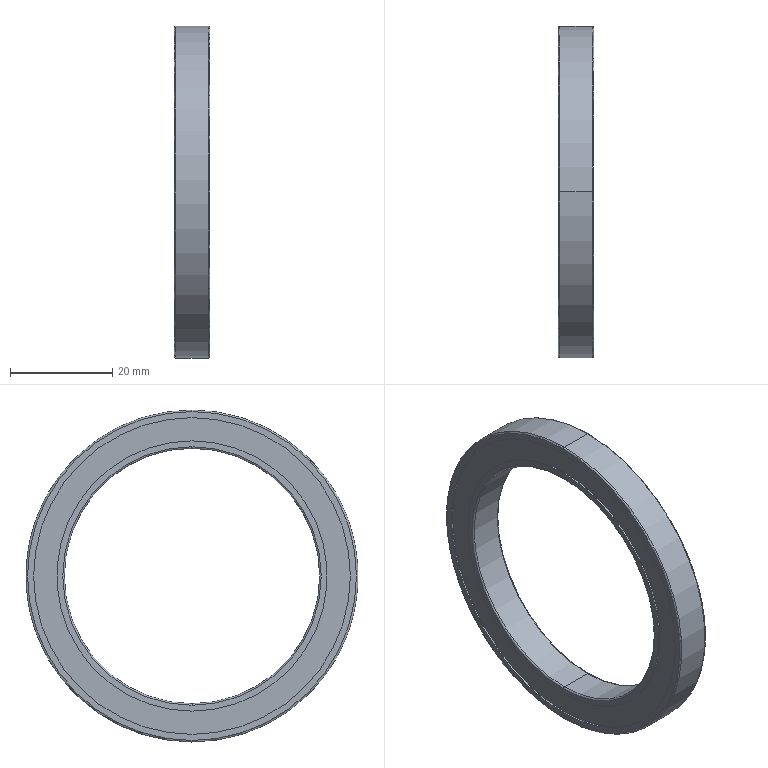Part | SolidWorks | features Fillet 2, Revolution 1 | 1 solid | 26 faces | box 7 x 65 x 65 mm | volume 8944 mm3 | cylinder 12 | torus 8 | plane 6 | commonest cylinder face diameters 52.9 x4 62 x4 50 x2 65 x2
STEP:
#1=CARTESIAN_POINT('',(0.3,0.,25.));
#2=VERTEX_POINT('',#1);
#3=CARTESIAN_POINT('',(0.3,0.,-25.));
#4=VERTEX_POINT('',#3);
#5=CARTESIAN_POINT('',(0.3,0.,0.));
#6=DIRECTION('',(-1.,0.,0.));
#7=DIRECTION('',(0.,0.,-1.));
#8=AXIS2_PLACEMENT_3D('',#5,#6,#7);
#9=CIRCLE('',#8,25.);
#10=EDGE_CURVE('',#2,#4,#9,.T.);
#11=ORIENTED_EDGE('',*,*,#10,.F.);
#12=CARTESIAN_POINT('',(0.,0.,25.3));
#13=VERTEX_POINT('',#12);
#14=CARTESIAN_POINT('',(0.3,0.,25.3));
#15=DIRECTION('',(0.,1.,0.));
#16=DIRECTION('',(0.,0.,1.));
#17=AXIS2_PLACEMENT_3D('',#14,#15,#16);
#18=CIRCLE('',#17,0.3);
#19=EDGE_CURVE('',#2,#13,#18,.T.);
#20=ORIENTED_EDGE('',*,*,#19,.T.);
#21=CARTESIAN_POINT('',(0.,0.,-25.3));
#22=VERTEX_POINT('',#21);
#23=CARTESIAN_POINT('',(0.,0.,0.));
#24=DIRECTION('',(1.,0.,0.));
#25=DIRECTION('',(0.,0.,-1.));
#26=AXIS2_PLACEMENT_3D('',#23,#24,#25);
#27=CIRCLE('',#26,25.3);
#28=EDGE_CURVE('',#22,#13,#27,.T.);
#29=ORIENTED_EDGE('',*,*,#28,.F.);
#30=CARTESIAN_POINT('',(0.3,0.,-25.3));
#31=DIRECTION('',(0.,-1.,0.));
#32=DIRECTION('',(0.,0.,-1.));
#33=AXIS2_PLACEMENT_3D('',#30,#31,#32);
#34=CIRCLE('',#33,0.3);
#35=EDGE_CURVE('',#4,#22,#34,.T.);
#36=ORIENTED_EDGE('',*,*,#35,.F.);
#37=EDGE_LOOP('',(#11,#20,#29,#36));
#38=FACE_OUTER_BOUND('',#37,.T.);
#39=CARTESIAN_POINT('',(0.3,0.,0.));
#40=DIRECTION('',(1.,0.,0.));
#41=DIRECTION('',(0.,0.,-1.));
#42=AXIS2_PLACEMENT_3D('',#39,#40,#41);
#43=TOROIDAL_SURFACE('',#42,25.3,0.3);
#44=ADVANCED_FACE('',(#38),#43,.T.);
#45=CARTESIAN_POINT('',(6.7,0.,-25.));
#46=VERTEX_POINT('',#45);
#47=CARTESIAN_POINT('',(6.7,0.,25.));
#48=VERTEX_POINT('',#47);
#49=CARTESIAN_POINT('',(6.7,0.,0.));
#50=DIRECTION('',(1.,0.,0.));
#51=DIRECTION('',(0.,0.,1.));
#52=AXIS2_PLACEMENT_3D('',#49,#50,#51);
#53=CIRCLE('',#52,25.);
#54=EDGE_CURVE('',#46,#48,#53,.T.);
#55=ORIENTED_EDGE('',*,*,#54,.F.);
#56=CARTESIAN_POINT('',(7.,0.,-25.3));
#57=VERTEX_POINT('',#56);
#58=CARTESIAN_POINT('',(6.7,0.,-25.3));
#59=DIRECTION('',(0.,1.,0.));
#60=DIRECTION('',(0.,0.,1.));
#61=AXIS2_PLACEMENT_3D('',#58,#59,#60);
#62=CIRCLE('',#61,0.3);
#63=EDGE_CURVE('',#46,#57,#62,.T.);
#64=ORIENTED_EDGE('',*,*,#63,.T.);
#65=CARTESIAN_POINT('',(7.,0.,25.3));
#66=VERTEX_POINT('',#65);
#67=CARTESIAN_POINT('',(7.,0.,0.));
#68=DIRECTION('',(-1.,0.,0.));
#69=DIRECTION('',(0.,0.,1.));
#70=AXIS2_PLACEMENT_3D('',#67,#68,#69);
#71=CIRCLE('',#70,25.3);
#72=EDGE_CURVE('',#66,#57,#71,.T.);
#73=ORIENTED_EDGE('',*,*,#72,.F.);
#74=CARTESIAN_POINT('',(6.7,0.,25.3));
#75=DIRECTION('',(0.,-1.,0.));
#76=DIRECTION('',(0.,0.,-1.));
#77=AXIS2_PLACEMENT_3D('',#74,#75,#76);
#78=CIRCLE('',#77,0.3);
#79=EDGE_CURVE('',#48,#66,#78,.T.);
#80=ORIENTED_EDGE('',*,*,#79,.F.);
#81=EDGE_LOOP('',(#55,#64,#73,#80));
#82=FACE_OUTER_BOUND('',#81,.T.);
#83=CARTESIAN_POINT('',(6.7,0.,0.));
#84=DIRECTION('',(-1.,0.,0.));
#85=DIRECTION('',(0.,0.,1.));
#86=AXIS2_PLACEMENT_3D('',#83,#84,#85);
#87=TOROIDAL_SURFACE('',#86,25.3,0.3);
#88=ADVANCED_FACE('',(#82),#87,.T.);
#89=CARTESIAN_POINT('',(0.,0.,32.2));
#90=VERTEX_POINT('',#89);
#91=CARTESIAN_POINT('',(0.,0.,-32.2));
#92=VERTEX_POINT('',#91);
#93=CARTESIAN_POINT('',(0.,0.,0.));
#94=DIRECTION('',(-1.,0.,0.));
#95=DIRECTION('',(0.,0.,-1.));
#96=AXIS2_PLACEMENT_3D('',#93,#94,#95);
#97=CIRCLE('',#96,32.2);
#98=EDGE_CURVE('',#90,#92,#97,.T.);
#99=ORIENTED_EDGE('',*,*,#98,.F.);
#100=CARTESIAN_POINT('',(0.3,0.,32.5));
#101=VERTEX_POINT('',#100);
#102=CARTESIAN_POINT('',(0.3,0.,32.2));
#103=DIRECTION('',(0.,1.,0.));
#104=DIRECTION('',(0.,0.,1.));
#105=AXIS2_PLACEMENT_3D('',#102,#103,#104);
#106=CIRCLE('',#105,0.3);
#107=EDGE_CURVE('',#90,#101,#106,.T.);
#108=ORIENTED_EDGE('',*,*,#107,.T.);
#109=CARTESIAN_POINT('',(0.3,0.,-32.5));
#110=VERTEX_POINT('',#109);
#111=CARTESIAN_POINT('',(0.3,0.,0.));
#112=DIRECTION('',(1.,0.,0.));
#113=DIRECTION('',(0.,0.,-1.));
#114=AXIS2_PLACEMENT_3D('',#111,#112,#113);
#115=CIRCLE('',#114,32.5);
#116=EDGE_CURVE('',#110,#101,#115,.T.);
#117=ORIENTED_EDGE('',*,*,#116,.F.);
#118=CARTESIAN_POINT('',(0.3,0.,-32.2));
#119=DIRECTION('',(0.,-1.,0.));
#120=DIRECTION('',(0.,0.,-1.));
#121=AXIS2_PLACEMENT_3D('',#118,#119,#120);
#122=CIRCLE('',#121,0.3);
#123=EDGE_CURVE('',#92,#110,#122,.T.);
#124=ORIENTED_EDGE('',*,*,#123,.F.);
#125=EDGE_LOOP('',(#99,#108,#117,#124));
#126=FACE_OUTER_BOUND('',#125,.T.);
#127=CARTESIAN_POINT('',(0.3,0.,0.));
#128=DIRECTION('',(1.,0.,0.));
#129=DIRECTION('',(0.,0.,-1.));
#130=AXIS2_PLACEMENT_3D('',#127,#128,#129);
#131=TOROIDAL_SURFACE('',#130,32.2,0.3);
#132=ADVANCED_FACE('',(#126),#131,.T.);
#133=CARTESIAN_POINT('',(7.,0.,-32.2));
#134=VERTEX_POINT('',#133);
#135=CARTESIAN_POINT('',(7.,0.,32.2));
#136=VERTEX_POINT('',#135);
#137=CARTESIAN_POINT('',(7.,0.,0.));
#138=DIRECTION('',(1.,0.,0.));
#139=DIRECTION('',(0.,0.,1.));
#140=AXIS2_PLACEMENT_3D('',#137,#138,#139);
#141=CIRCLE('',#140,32.2);
#142=EDGE_CURVE('',#134,#136,#141,.T.);
#143=ORIENTED_EDGE('',*,*,#142,.F.);
#144=CARTESIAN_POINT('',(6.7,0.,-32.5));
#145=VERTEX_POINT('',#144);
#146=CARTESIAN_POINT('',(6.7,0.,-32.2));
#147=DIRECTION('',(0.,1.,0.));
#148=DIRECTION('',(0.,0.,1.));
#149=AXIS2_PLACEMENT_3D('',#146,#147,#148);
#150=CIRCLE('',#149,0.3);
#151=EDGE_CURVE('',#134,#145,#150,.T.);
#152=ORIENTED_EDGE('',*,*,#151,.T.);
#153=CARTESIAN_POINT('',(6.7,0.,32.5));
#154=VERTEX_POINT('',#153);
#155=CARTESIAN_POINT('',(6.7,0.,0.));
#156=DIRECTION('',(-1.,0.,0.));
#157=DIRECTION('',(0.,0.,1.));
#158=AXIS2_PLACEMENT_3D('',#155,#156,#157);
#159=CIRCLE('',#158,32.5);
#160=EDGE_CURVE('',#154,#145,#159,.T.);
#161=ORIENTED_EDGE('',*,*,#160,.F.);
#162=CARTESIAN_POINT('',(6.7,0.,32.2));
#163=DIRECTION('',(0.,-1.,0.));
#164=DIRECTION('',(0.,0.,-1.));
#165=AXIS2_PLACEMENT_3D('',#162,#163,#164);
#166=CIRCLE('',#165,0.3);
#167=EDGE_CURVE('',#136,#154,#166,.T.);
#168=ORIENTED_EDGE('',*,*,#167,.F.);
#169=EDGE_LOOP('',(#143,#152,#161,#168));
#170=FACE_OUTER_BOUND('',#169,.T.);
#171=CARTESIAN_POINT('',(6.7,0.,0.));
#172=DIRECTION('',(-1.,0.,0.));
#173=DIRECTION('',(0.,0.,1.));
#174=AXIS2_PLACEMENT_3D('',#171,#172,#173);
#175=TOROIDAL_SURFACE('',#174,32.2,0.3);
#176=ADVANCED_FACE('',(#170),#175,.T.);
#177=ORIENTED_EDGE('',*,*,#160,.T.);
#178=CARTESIAN_POINT('',(0.,0.,-32.5));
#179=DIRECTION('',(-1.,0.,0.));
#180=VECTOR('',#179,1000.);
#181=LINE('',#178,#180);
#182=EDGE_CURVE('',#145,#110,#181,.T.);
#183=ORIENTED_EDGE('',*,*,#182,.T.);
#184=ORIENTED_EDGE('',*,*,#116,.T.);
#185=CARTESIAN_POINT('',(0.,0.,32.5));
#186=DIRECTION('',(-1.,0.,0.));
#187=VECTOR('',#186,1000.);
#188=LINE('',#185,#187);
#189=EDGE_CURVE('',#154,#101,#188,.T.);
#190=ORIENTED_EDGE('',*,*,#189,.F.);
#191=EDGE_LOOP('',(#177,#183,#184,#190));
#192=FACE_OUTER_BOUND('',#191,.T.);
#193=CARTESIAN_POINT('',(0.,0.,0.));
#194=DIRECTION('',(-1.,0.,0.));
#195=DIRECTION('',(0.,0.,1.));
#196=AXIS2_PLACEMENT_3D('',#193,#194,#195);
#197=CYLINDRICAL_SURFACE('',#196,32.5);
#198=ADVANCED_FACE('',(#192),#197,.T.);
#199=CARTESIAN_POINT('',(7.,0.,-31.));
#200=VERTEX_POINT('',#199);
#201=CARTESIAN_POINT('',(7.,0.,31.));
#202=VERTEX_POINT('',#201);
#203=CARTESIAN_POINT('',(7.,0.,0.));
#204=DIRECTION('',(-1.,0.,0.));
#205=DIRECTION('',(0.,0.,1.));
#206=AXIS2_PLACEMENT_3D('',#203,#204,#205);
#207=CIRCLE('',#206,31.);
#208=EDGE_CURVE('',#200,#202,#207,.T.);
#209=ORIENTED_EDGE('',*,*,#208,.F.);
#210=CARTESIAN_POINT('',(6.68,0.,-31.));
#211=VERTEX_POINT('',#210);
#212=CARTESIAN_POINT('',(0.,0.,-31.));
#213=DIRECTION('',(-1.,0.,0.));
#214=VECTOR('',#213,1000.);
#215=LINE('',#212,#214);
#216=EDGE_CURVE('',#200,#211,#215,.T.);
#217=ORIENTED_EDGE('',*,*,#216,.T.);
#218=CARTESIAN_POINT('',(6.68,0.,31.));
#219=VERTEX_POINT('',#218);
#220=CARTESIAN_POINT('',(6.68,0.,0.));
#221=DIRECTION('',(-1.,0.,0.));
#222=DIRECTION('',(0.,0.,1.));
#223=AXIS2_PLACEMENT_3D('',#220,#221,#222);
#224=CIRCLE('',#223,31.);
#225=EDGE_CURVE('',#211,#219,#224,.T.);
#226=ORIENTED_EDGE('',*,*,#225,.T.);
#227=CARTESIAN_POINT('',(0.,0.,31.));
#228=DIRECTION('',(-1.,0.,0.));
#229=VECTOR('',#228,1000.);
#230=LINE('',#227,#229);
#231=EDGE_CURVE('',#202,#219,#230,.T.);
#232=ORIENTED_EDGE('',*,*,#231,.F.);
#233=EDGE_LOOP('',(#209,#217,#226,#232));
#234=FACE_OUTER_BOUND('',#233,.T.);
#235=CARTESIAN_POINT('',(0.,0.,0.));
#236=DIRECTION('',(-1.,0.,0.));
#237=DIRECTION('',(0.,0.,1.));
#238=AXIS2_PLACEMENT_3D('',#235,#236,#237);
#239=CYLINDRICAL_SURFACE('',#238,31.);
#240=ADVANCED_FACE('',(#234),#239,.F.);
#241=CARTESIAN_POINT('',(7.,0.,26.45));
#242=VERTEX_POINT('',#241);
#243=CARTESIAN_POINT('',(7.,0.,-26.45));
#244=VERTEX_POINT('',#243);
#245=CARTESIAN_POINT('',(7.,0.,0.));
#246=DIRECTION('',(-1.,0.,0.));
#247=DIRECTION('',(0.,0.,1.));
#248=AXIS2_PLACEMENT_3D('',#245,#246,#247);
#249=CIRCLE('',#248,26.45);
#250=EDGE_CURVE('',#242,#244,#249,.T.);
#251=ORIENTED_EDGE('',*,*,#250,.T.);
#252=CARTESIAN_POINT('',(6.68,0.,-26.45));
#253=VERTEX_POINT('',#252);
#254=CARTESIAN_POINT('',(0.,0.,-26.45));
#255=DIRECTION('',(-1.,0.,0.));
#256=VECTOR('',#255,1000.);
#257=LINE('',#254,#256);
#258=EDGE_CURVE('',#244,#253,#257,.T.);
#259=ORIENTED_EDGE('',*,*,#258,.T.);
#260=CARTESIAN_POINT('',(6.68,0.,26.45));
#261=VERTEX_POINT('',#260);
#262=CARTESIAN_POINT('',(6.68,0.,0.));
#263=DIRECTION('',(-1.,0.,0.));
#264=DIRECTION('',(0.,0.,1.));
#265=AXIS2_PLACEMENT_3D('',#262,#263,#264);
#266=CIRCLE('',#265,26.45);
#267=EDGE_CURVE('',#261,#253,#266,.T.);
#268=ORIENTED_EDGE('',*,*,#267,.F.);
#269=CARTESIAN_POINT('',(0.,0.,26.45));
#270=DIRECTION('',(-1.,0.,0.));
#271=VECTOR('',#270,1000.);
#272=LINE('',#269,#271);
#273=EDGE_CURVE('',#242,#261,#272,.T.);
#274=ORIENTED_EDGE('',*,*,#273,.F.);
#275=EDGE_LOOP('',(#251,#259,#268,#274));
#276=FACE_OUTER_BOUND('',#275,.T.);
#277=CARTESIAN_POINT('',(0.,0.,0.));
#278=DIRECTION('',(-1.,0.,0.));
#279=DIRECTION('',(0.,0.,1.));
#280=AXIS2_PLACEMENT_3D('',#277,#278,#279);
#281=CYLINDRICAL_SURFACE('',#280,26.45);
#282=ADVANCED_FACE('',(#276),#281,.T.);
#283=CARTESIAN_POINT('',(6.7,0.,0.));
#284=DIRECTION('',(1.,0.,0.));
#285=DIRECTION('',(0.,0.,1.));
#286=AXIS2_PLACEMENT_3D('',#283,#284,#285);
#287=CIRCLE('',#286,25.);
#288=EDGE_CURVE('',#48,#46,#287,.T.);
#289=ORIENTED_EDGE('',*,*,#288,.T.);
#290=CARTESIAN_POINT('',(0.,0.,-25.));
#291=DIRECTION('',(-1.,0.,0.));
#292=VECTOR('',#291,1000.);
#293=LINE('',#290,#292);
#294=EDGE_CURVE('',#46,#4,#293,.T.);
#295=ORIENTED_EDGE('',*,*,#294,.T.);
#296=CARTESIAN_POINT('',(0.3,0.,0.));
#297=DIRECTION('',(-1.,0.,0.));
#298=DIRECTION('',(0.,0.,-1.));
#299=AXIS2_PLACEMENT_3D('',#296,#297,#298);
#300=CIRCLE('',#299,25.);
#301=EDGE_CURVE('',#4,#2,#300,.T.);
#302=ORIENTED_EDGE('',*,*,#301,.T.);
#303=CARTESIAN_POINT('',(0.,0.,25.));
#304=DIRECTION('',(-1.,0.,0.));
#305=VECTOR('',#304,1000.);
#306=LINE('',#303,#305);
#307=EDGE_CURVE('',#48,#2,#306,.T.);
#308=ORIENTED_EDGE('',*,*,#307,.F.);
#309=EDGE_LOOP('',(#289,#295,#302,#308));
#310=FACE_OUTER_BOUND('',#309,.T.);
#311=CARTESIAN_POINT('',(0.,0.,0.));
#312=DIRECTION('',(-1.,0.,0.));
#313=DIRECTION('',(0.,0.,1.));
#314=AXIS2_PLACEMENT_3D('',#311,#312,#313);
#315=CYLINDRICAL_SURFACE('',#314,25.);
#316=ADVANCED_FACE('',(#310),#315,.F.);
#317=CARTESIAN_POINT('',(0.32,0.,26.45));
#318=VERTEX_POINT('',#317);
#319=CARTESIAN_POINT('',(0.32,0.,-26.45));
#320=VERTEX_POINT('',#319);
#321=CARTESIAN_POINT('',(0.32,0.,0.));
#322=DIRECTION('',(-1.,0.,0.));
#323=DIRECTION('',(0.,0.,1.));
#324=AXIS2_PLACEMENT_3D('',#321,#322,#323);
#325=CIRCLE('',#324,26.45);
#326=EDGE_CURVE('',#318,#320,#325,.T.);
#327=ORIENTED_EDGE('',*,*,#326,.T.);
#328=CARTESIAN_POINT('',(0.,0.,-26.45));
#329=VERTEX_POINT('',#328);
#330=CARTESIAN_POINT('',(0.,0.,-26.45));
#331=DIRECTION('',(-1.,0.,0.));
#332=VECTOR('',#331,1000.);
#333=LINE('',#330,#332);
#334=EDGE_CURVE('',#320,#329,#333,.T.);
#335=ORIENTED_EDGE('',*,*,#334,.T.);
#336=CARTESIAN_POINT('',(0.,0.,26.45));
#337=VERTEX_POINT('',#336);
#338=CARTESIAN_POINT('',(0.,0.,0.));
#339=DIRECTION('',(-1.,0.,0.));
#340=DIRECTION('',(0.,0.,1.));
#341=AXIS2_PLACEMENT_3D('',#338,#339,#340);
#342=CIRCLE('',#341,26.45);
#343=EDGE_CURVE('',#337,#329,#342,.T.);
#344=ORIENTED_EDGE('',*,*,#343,.F.);
#345=CARTESIAN_POINT('',(0.,0.,26.45));
#346=DIRECTION('',(-1.,0.,0.));
#347=VECTOR('',#346,1000.);
#348=LINE('',#345,#347);
#349=EDGE_CURVE('',#318,#337,#348,.T.);
#350=ORIENTED_EDGE('',*,*,#349,.F.);
#351=EDGE_LOOP('',(#327,#335,#344,#350));
#352=FACE_OUTER_BOUND('',#351,.T.);
#353=CARTESIAN_POINT('',(0.,0.,0.));
#354=DIRECTION('',(-1.,0.,0.));
#355=DIRECTION('',(0.,0.,1.));
#356=AXIS2_PLACEMENT_3D('',#353,#354,#355);
#357=CYLINDRICAL_SURFACE('',#356,26.45);
#358=ADVANCED_FACE('',(#352),#357,.T.);
#359=CARTESIAN_POINT('',(0.32,0.,-31.));
#360=VERTEX_POINT('',#359);
#361=CARTESIAN_POINT('',(0.32,0.,31.));
#362=VERTEX_POINT('',#361);
#363=CARTESIAN_POINT('',(0.32,0.,0.));
#364=DIRECTION('',(-1.,0.,0.));
#365=DIRECTION('',(0.,0.,1.));
#366=AXIS2_PLACEMENT_3D('',#363,#364,#365);
#367=CIRCLE('',#366,31.);
#368=EDGE_CURVE('',#360,#362,#367,.T.);
#369=ORIENTED_EDGE('',*,*,#368,.F.);
#370=CARTESIAN_POINT('',(0.,0.,-31.));
#371=VERTEX_POINT('',#370);
#372=CARTESIAN_POINT('',(0.,0.,-31.));
#373=DIRECTION('',(-1.,0.,0.));
#374=VECTOR('',#373,1000.);
#375=LINE('',#372,#374);
#376=EDGE_CURVE('',#360,#371,#375,.T.);
#377=ORIENTED_EDGE('',*,*,#376,.T.);
#378=CARTESIAN_POINT('',(0.,0.,31.));
#379=VERTEX_POINT('',#378);
#380=CARTESIAN_POINT('',(0.,0.,0.));
#381=DIRECTION('',(-1.,0.,0.));
#382=DIRECTION('',(0.,0.,1.));
#383=AXIS2_PLACEMENT_3D('',#380,#381,#382);
#384=CIRCLE('',#383,31.);
#385=EDGE_CURVE('',#371,#379,#384,.T.);
#386=ORIENTED_EDGE('',*,*,#385,.T.);
#387=CARTESIAN_POINT('',(0.,0.,31.));
#388=DIRECTION('',(-1.,0.,0.));
#389=VECTOR('',#388,1000.);
#390=LINE('',#387,#389);
#391=EDGE_CURVE('',#362,#379,#390,.T.);
#392=ORIENTED_EDGE('',*,*,#391,.F.);
#393=EDGE_LOOP('',(#369,#377,#386,#392));
#394=FACE_OUTER_BOUND('',#393,.T.);
#395=CARTESIAN_POINT('',(0.,0.,0.));
#396=DIRECTION('',(-1.,0.,0.));
#397=DIRECTION('',(0.,0.,1.));
#398=AXIS2_PLACEMENT_3D('',#395,#396,#397);
#399=CYLINDRICAL_SURFACE('',#398,31.);
#400=ADVANCED_FACE('',(#394),#399,.F.);
#401=CARTESIAN_POINT('',(0.,0.,0.));
#402=DIRECTION('',(-1.,0.,0.));
#403=DIRECTION('',(0.,0.,-1.));
#404=AXIS2_PLACEMENT_3D('',#401,#402,#403);
#405=CIRCLE('',#404,32.2);
#406=EDGE_CURVE('',#92,#90,#405,.T.);
#407=ORIENTED_EDGE('',*,*,#406,.T.);
#408=ORIENTED_EDGE('',*,*,#98,.T.);
#409=EDGE_LOOP('',(#407,#408));
#410=FACE_OUTER_BOUND('',#409,.T.);
#411=CARTESIAN_POINT('',(0.,0.,0.));
#412=DIRECTION('',(-1.,0.,0.));
#413=DIRECTION('',(0.,0.,1.));
#414=AXIS2_PLACEMENT_3D('',#411,#412,#413);
#415=CIRCLE('',#414,31.);
#416=EDGE_CURVE('',#379,#371,#415,.T.);
#417=ORIENTED_EDGE('',*,*,#416,.F.);
#418=ORIENTED_EDGE('',*,*,#385,.F.);
#419=EDGE_LOOP('',(#417,#418));
#420=FACE_BOUND('',#419,.T.);
#421=CARTESIAN_POINT('',(0.,32.5,0.));
#422=DIRECTION('',(1.,0.,0.));
#423=DIRECTION('',(0.,0.,-1.));
#424=AXIS2_PLACEMENT_3D('',#421,#422,#423);
#425=PLANE('',#424);
#426=ADVANCED_FACE('',(#410,#420),#425,.F.);
#427=ORIENTED_EDGE('',*,*,#376,.F.);
#428=CARTESIAN_POINT('',(0.32,0.,0.));
#429=DIRECTION('',(-1.,0.,0.));
#430=DIRECTION('',(0.,0.,1.));
#431=AXIS2_PLACEMENT_3D('',#428,#429,#430);
#432=CIRCLE('',#431,31.);
#433=EDGE_CURVE('',#362,#360,#432,.T.);
#434=ORIENTED_EDGE('',*,*,#433,.F.);
#435=ORIENTED_EDGE('',*,*,#391,.T.);
#436=ORIENTED_EDGE('',*,*,#416,.T.);
#437=EDGE_LOOP('',(#427,#434,#435,#436));
#438=FACE_OUTER_BOUND('',#437,.T.);
#439=CARTESIAN_POINT('',(0.,0.,0.));
#440=DIRECTION('',(-1.,0.,0.));
#441=DIRECTION('',(0.,0.,1.));
#442=AXIS2_PLACEMENT_3D('',#439,#440,#441);
#443=CYLINDRICAL_SURFACE('',#442,31.);
#444=ADVANCED_FACE('',(#438),#443,.F.);
#445=ORIENTED_EDGE('',*,*,#326,.F.);
#446=CARTESIAN_POINT('',(0.32,0.,0.));
#447=DIRECTION('',(-1.,0.,0.));
#448=DIRECTION('',(0.,0.,1.));
#449=AXIS2_PLACEMENT_3D('',#446,#447,#448);
#450=CIRCLE('',#449,26.45);
#451=EDGE_CURVE('',#320,#318,#450,.T.);
#452=ORIENTED_EDGE('',*,*,#451,.F.);
#453=EDGE_LOOP('',(#445,#452));
#454=FACE_BOUND('',#453,.T.);
#455=ORIENTED_EDGE('',*,*,#433,.T.);
#456=ORIENTED_EDGE('',*,*,#368,.T.);
#457=EDGE_LOOP('',(#455,#456));
#458=FACE_OUTER_BOUND('',#457,.T.);
#459=CARTESIAN_POINT('',(0.32,31.,0.));
#460=DIRECTION('',(1.,0.,0.));
#461=DIRECTION('',(0.,0.,-1.));
#462=AXIS2_PLACEMENT_3D('',#459,#460,#461);
#463=PLANE('',#462);
#464=ADVANCED_FACE('',(#454,#458),#463,.F.);
#465=ORIENTED_EDGE('',*,*,#334,.F.);
#466=ORIENTED_EDGE('',*,*,#451,.T.);
#467=ORIENTED_EDGE('',*,*,#349,.T.);
#468=CARTESIAN_POINT('',(0.,0.,0.));
#469=DIRECTION('',(-1.,0.,0.));
#470=DIRECTION('',(0.,0.,1.));
#471=AXIS2_PLACEMENT_3D('',#468,#469,#470);
#472=CIRCLE('',#471,26.45);
#473=EDGE_CURVE('',#329,#337,#472,.T.);
#474=ORIENTED_EDGE('',*,*,#473,.F.);
#475=EDGE_LOOP('',(#465,#466,#467,#474));
#476=FACE_OUTER_BOUND('',#475,.T.);
#477=CARTESIAN_POINT('',(0.,0.,0.));
#478=DIRECTION('',(-1.,0.,0.));
#479=DIRECTION('',(0.,0.,1.));
#480=AXIS2_PLACEMENT_3D('',#477,#478,#479);
#481=CYLINDRICAL_SURFACE('',#480,26.45);
#482=ADVANCED_FACE('',(#476),#481,.T.);
#483=ORIENTED_EDGE('',*,*,#28,.T.);
#484=CARTESIAN_POINT('',(0.,0.,0.));
#485=DIRECTION('',(1.,0.,0.));
#486=DIRECTION('',(0.,0.,-1.));
#487=AXIS2_PLACEMENT_3D('',#484,#485,#486);
#488=CIRCLE('',#487,25.3);
#489=EDGE_CURVE('',#13,#22,#488,.T.);
#490=ORIENTED_EDGE('',*,*,#489,.T.);
#491=EDGE_LOOP('',(#483,#490));
#492=FACE_BOUND('',#491,.T.);
#493=ORIENTED_EDGE('',*,*,#343,.T.);
#494=ORIENTED_EDGE('',*,*,#473,.T.);
#495=EDGE_LOOP('',(#493,#494));
#496=FACE_OUTER_BOUND('',#495,.T.);
#497=CARTESIAN_POINT('',(0.,26.45,0.));
#498=DIRECTION('',(1.,0.,0.));
#499=DIRECTION('',(0.,0.,-1.));
#500=AXIS2_PLACEMENT_3D('',#497,#498,#499);
#501=PLANE('',#500);
#502=ADVANCED_FACE('',(#492,#496),#501,.F.);
#503=ORIENTED_EDGE('',*,*,#294,.F.);
#504=ORIENTED_EDGE('',*,*,#54,.T.);
#505=ORIENTED_EDGE('',*,*,#307,.T.);
#506=ORIENTED_EDGE('',*,*,#10,.T.);
#507=EDGE_LOOP('',(#503,#504,#505,#506));
#508=FACE_OUTER_BOUND('',#507,.T.);
#509=CARTESIAN_POINT('',(0.,0.,0.));
#510=DIRECTION('',(-1.,0.,0.));
#511=DIRECTION('',(0.,0.,1.));
#512=AXIS2_PLACEMENT_3D('',#509,#510,#511);
#513=CYLINDRICAL_SURFACE('',#512,25.);
#514=ADVANCED_FACE('',(#508),#513,.F.);
#515=ORIENTED_EDGE('',*,*,#72,.T.);
#516=CARTESIAN_POINT('',(7.,0.,0.));
#517=DIRECTION('',(-1.,0.,0.));
#518=DIRECTION('',(0.,0.,1.));
#519=AXIS2_PLACEMENT_3D('',#516,#517,#518);
#520=CIRCLE('',#519,25.3);
#521=EDGE_CURVE('',#57,#66,#520,.T.);
#522=ORIENTED_EDGE('',*,*,#521,.T.);
#523=EDGE_LOOP('',(#515,#522));
#524=FACE_BOUND('',#523,.T.);
#525=ORIENTED_EDGE('',*,*,#250,.F.);
#526=CARTESIAN_POINT('',(7.,0.,0.));
#527=DIRECTION('',(-1.,0.,0.));
#528=DIRECTION('',(0.,0.,1.));
#529=AXIS2_PLACEMENT_3D('',#526,#527,#528);
#530=CIRCLE('',#529,26.45);
#531=EDGE_CURVE('',#244,#242,#530,.T.);
#532=ORIENTED_EDGE('',*,*,#531,.F.);
#533=EDGE_LOOP('',(#525,#532));
#534=FACE_OUTER_BOUND('',#533,.T.);
#535=CARTESIAN_POINT('',(7.,26.45,0.));
#536=DIRECTION('',(-1.,0.,0.));
#537=DIRECTION('',(0.,0.,1.));
#538=AXIS2_PLACEMENT_3D('',#535,#536,#537);
#539=PLANE('',#538);
#540=ADVANCED_FACE('',(#524,#534),#539,.F.);
#541=ORIENTED_EDGE('',*,*,#258,.F.);
#542=ORIENTED_EDGE('',*,*,#531,.T.);
#543=ORIENTED_EDGE('',*,*,#273,.T.);
#544=CARTESIAN_POINT('',(6.68,0.,0.));
#545=DIRECTION('',(-1.,0.,0.));
#546=DIRECTION('',(0.,0.,1.));
#547=AXIS2_PLACEMENT_3D('',#544,#545,#546);
#548=CIRCLE('',#547,26.45);
#549=EDGE_CURVE('',#253,#261,#548,.T.);
#550=ORIENTED_EDGE('',*,*,#549,.F.);
#551=EDGE_LOOP('',(#541,#542,#543,#550));
#552=FACE_OUTER_BOUND('',#551,.T.);
#553=CARTESIAN_POINT('',(0.,0.,0.));
#554=DIRECTION('',(-1.,0.,0.));
#555=DIRECTION('',(0.,0.,1.));
#556=AXIS2_PLACEMENT_3D('',#553,#554,#555);
#557=CYLINDRICAL_SURFACE('',#556,26.45);
#558=ADVANCED_FACE('',(#552),#557,.T.);
#559=CARTESIAN_POINT('',(6.68,0.,0.));
#560=DIRECTION('',(-1.,0.,0.));
#561=DIRECTION('',(0.,0.,1.));
#562=AXIS2_PLACEMENT_3D('',#559,#560,#561);
#563=CIRCLE('',#562,31.);
#564=EDGE_CURVE('',#219,#211,#563,.T.);
#565=ORIENTED_EDGE('',*,*,#564,.F.);
#566=ORIENTED_EDGE('',*,*,#225,.F.);
#567=EDGE_LOOP('',(#565,#566));
#568=FACE_OUTER_BOUND('',#567,.T.);
#569=ORIENTED_EDGE('',*,*,#267,.T.);
#570=ORIENTED_EDGE('',*,*,#549,.T.);
#571=EDGE_LOOP('',(#569,#570));
#572=FACE_BOUND('',#571,.T.);
#573=CARTESIAN_POINT('',(6.68,31.,0.));
#574=DIRECTION('',(-1.,0.,0.));
#575=DIRECTION('',(0.,0.,1.));
#576=AXIS2_PLACEMENT_3D('',#573,#574,#575);
#577=PLANE('',#576);
#578=ADVANCED_FACE('',(#568,#572),#577,.F.);
#579=ORIENTED_EDGE('',*,*,#216,.F.);
#580=CARTESIAN_POINT('',(7.,0.,0.));
#581=DIRECTION('',(-1.,0.,0.));
#582=DIRECTION('',(0.,0.,1.));
#583=AXIS2_PLACEMENT_3D('',#580,#581,#582);
#584=CIRCLE('',#583,31.);
#585=EDGE_CURVE('',#202,#200,#584,.T.);
#586=ORIENTED_EDGE('',*,*,#585,.F.);
#587=ORIENTED_EDGE('',*,*,#231,.T.);
#588=ORIENTED_EDGE('',*,*,#564,.T.);
#589=EDGE_LOOP('',(#579,#586,#587,#588));
#590=FACE_OUTER_BOUND('',#589,.T.);
#591=CARTESIAN_POINT('',(0.,0.,0.));
#592=DIRECTION('',(-1.,0.,0.));
#593=DIRECTION('',(0.,0.,1.));
#594=AXIS2_PLACEMENT_3D('',#591,#592,#593);
#595=CYLINDRICAL_SURFACE('',#594,31.);
#596=ADVANCED_FACE('',(#590),#595,.F.);
#597=CARTESIAN_POINT('',(7.,0.,0.));
#598=DIRECTION('',(1.,0.,0.));
#599=DIRECTION('',(0.,0.,1.));
#600=AXIS2_PLACEMENT_3D('',#597,#598,#599);
#601=CIRCLE('',#600,32.2);
#602=EDGE_CURVE('',#136,#134,#601,.T.);
#603=ORIENTED_EDGE('',*,*,#602,.T.);
#604=ORIENTED_EDGE('',*,*,#142,.T.);
#605=EDGE_LOOP('',(#603,#604));
#606=FACE_OUTER_BOUND('',#605,.T.);
#607=ORIENTED_EDGE('',*,*,#585,.T.);
#608=ORIENTED_EDGE('',*,*,#208,.T.);
#609=EDGE_LOOP('',(#607,#608));
#610=FACE_BOUND('',#609,.T.);
#611=CARTESIAN_POINT('',(7.,32.5,0.));
#612=DIRECTION('',(-1.,0.,0.));
#613=DIRECTION('',(0.,0.,1.));
#614=AXIS2_PLACEMENT_3D('',#611,#612,#613);
#615=PLANE('',#614);
#616=ADVANCED_FACE('',(#606,#610),#615,.F.);
#617=ORIENTED_EDGE('',*,*,#182,.F.);
#618=CARTESIAN_POINT('',(6.7,0.,0.));
#619=DIRECTION('',(-1.,0.,0.));
#620=DIRECTION('',(0.,0.,1.));
#621=AXIS2_PLACEMENT_3D('',#618,#619,#620);
#622=CIRCLE('',#621,32.5);
#623=EDGE_CURVE('',#145,#154,#622,.T.);
#624=ORIENTED_EDGE('',*,*,#623,.T.);
#625=ORIENTED_EDGE('',*,*,#189,.T.);
#626=CARTESIAN_POINT('',(0.3,0.,0.));
#627=DIRECTION('',(1.,0.,0.));
#628=DIRECTION('',(0.,0.,-1.));
#629=AXIS2_PLACEMENT_3D('',#626,#627,#628);
#630=CIRCLE('',#629,32.5);
#631=EDGE_CURVE('',#101,#110,#630,.T.);
#632=ORIENTED_EDGE('',*,*,#631,.T.);
#633=EDGE_LOOP('',(#617,#624,#625,#632));
#634=FACE_OUTER_BOUND('',#633,.T.);
#635=CARTESIAN_POINT('',(0.,0.,0.));
#636=DIRECTION('',(-1.,0.,0.));
#637=DIRECTION('',(0.,0.,1.));
#638=AXIS2_PLACEMENT_3D('',#635,#636,#637);
#639=CYLINDRICAL_SURFACE('',#638,32.5);
#640=ADVANCED_FACE('',(#634),#639,.T.);
#641=ORIENTED_EDGE('',*,*,#151,.F.);
#642=ORIENTED_EDGE('',*,*,#602,.F.);
#643=ORIENTED_EDGE('',*,*,#167,.T.);
#644=ORIENTED_EDGE('',*,*,#623,.F.);
#645=EDGE_LOOP('',(#641,#642,#643,#644));
#646=FACE_OUTER_BOUND('',#645,.T.);
#647=CARTESIAN_POINT('',(6.7,0.,0.));
#648=DIRECTION('',(-1.,0.,0.));
#649=DIRECTION('',(0.,0.,1.));
#650=AXIS2_PLACEMENT_3D('',#647,#648,#649);
#651=TOROIDAL_SURFACE('',#650,32.2,0.3);
#652=ADVANCED_FACE('',(#646),#651,.T.);
#653=ORIENTED_EDGE('',*,*,#107,.F.);
#654=ORIENTED_EDGE('',*,*,#406,.F.);
#655=ORIENTED_EDGE('',*,*,#123,.T.);
#656=ORIENTED_EDGE('',*,*,#631,.F.);
#657=EDGE_LOOP('',(#653,#654,#655,#656));
#658=FACE_OUTER_BOUND('',#657,.T.);
#659=CARTESIAN_POINT('',(0.3,0.,0.));
#660=DIRECTION('',(1.,0.,0.));
#661=DIRECTION('',(0.,0.,-1.));
#662=AXIS2_PLACEMENT_3D('',#659,#660,#661);
#663=TOROIDAL_SURFACE('',#662,32.2,0.3);
#664=ADVANCED_FACE('',(#658),#663,.T.);
#665=ORIENTED_EDGE('',*,*,#63,.F.);
#666=ORIENTED_EDGE('',*,*,#288,.F.);
#667=ORIENTED_EDGE('',*,*,#79,.T.);
#668=ORIENTED_EDGE('',*,*,#521,.F.);
#669=EDGE_LOOP('',(#665,#666,#667,#668));
#670=FACE_OUTER_BOUND('',#669,.T.);
#671=CARTESIAN_POINT('',(6.7,0.,0.));
#672=DIRECTION('',(-1.,0.,0.));
#673=DIRECTION('',(0.,0.,1.));
#674=AXIS2_PLACEMENT_3D('',#671,#672,#673);
#675=TOROIDAL_SURFACE('',#674,25.3,0.3);
#676=ADVANCED_FACE('',(#670),#675,.T.);
#677=ORIENTED_EDGE('',*,*,#19,.F.);
#678=ORIENTED_EDGE('',*,*,#301,.F.);
#679=ORIENTED_EDGE('',*,*,#35,.T.);
#680=ORIENTED_EDGE('',*,*,#489,.F.);
#681=EDGE_LOOP('',(#677,#678,#679,#680));
#682=FACE_OUTER_BOUND('',#681,.T.);
#683=CARTESIAN_POINT('',(0.3,0.,0.));
#684=DIRECTION('',(1.,0.,0.));
#685=DIRECTION('',(0.,0.,-1.));
#686=AXIS2_PLACEMENT_3D('',#683,#684,#685);
#687=TOROIDAL_SURFACE('',#686,25.3,0.3);
#688=ADVANCED_FACE('',(#682),#687,.T.);
#689=CLOSED_SHELL('',(#44,#88,#132,#176,#198,#240,#282,#316,#358,#400,#426,#444,#464,#482,#502,#514,#540,#558,#578,#596,#616,#640,#652,#664,#676,#688));
#690=MANIFOLD_SOLID_BREP('',#689);
#691=CARTESIAN_POINT('',(0.,0.,0.));
#692=DIRECTION('',(0.,0.,1.));
#693=DIRECTION('',(1.,0.,0.));
#694=AXIS2_PLACEMENT_3D('',#691,#692,#693);
#695=(LENGTH_UNIT()NAMED_UNIT(*)SI_UNIT(.MILLI.,.METRE.));
#696=UNCERTAINTY_MEASURE_WITH_UNIT(LENGTH_MEASURE(0.00001),#695,'','');
#697=(NAMED_UNIT(*)PLANE_ANGLE_UNIT()SI_UNIT($,.RADIAN.));
#698=(NAMED_UNIT(*)SI_UNIT($,.STERADIAN.)SOLID_ANGLE_UNIT());
#699=(GEOMETRIC_REPRESENTATION_CONTEXT(3)GLOBAL_UNCERTAINTY_ASSIGNED_CONTEXT((#696))GLOBAL_UNIT_ASSIGNED_CONTEXT((#695,#697,#698))REPRESENTATION_CONTEXT('',''));
#700=ADVANCED_BREP_SHAPE_REPRESENTATION('',(#690,#694),#699);